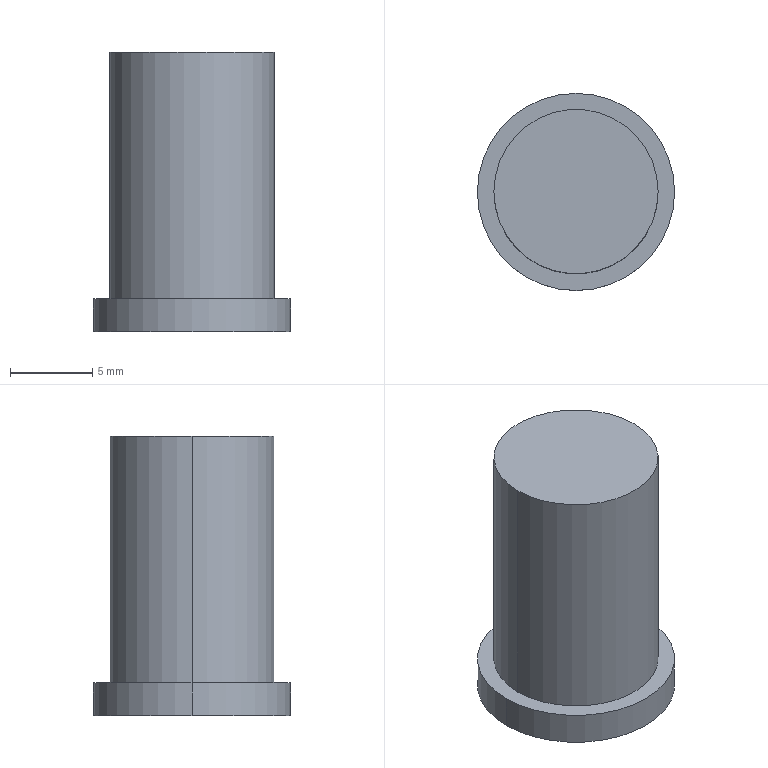Part | SolidWorks | features Extrusion 1, ICE 1 | 1 solid | 7 faces | box 12 x 12 x 17 mm | volume 1404 mm3 | cylinder 4 | plane 3 | commonest cylinder face diameters 10 x2 12 x2
STEP:
#1=CARTESIAN_POINT('',(5.,0.,17.));
#2=VERTEX_POINT('',#1);
#3=CARTESIAN_POINT('',(-5.,0.,17.));
#4=VERTEX_POINT('',#3);
#5=CARTESIAN_POINT('',(0.,0.,17.));
#6=DIRECTION('',(0.,0.,1.));
#7=DIRECTION('',(1.,0.,0.));
#8=AXIS2_PLACEMENT_3D('',#5,#6,#7);
#9=CIRCLE('',#8,5.);
#10=EDGE_CURVE('',#2,#4,#9,.T.);
#11=ORIENTED_EDGE('',*,*,#10,.F.);
#12=CARTESIAN_POINT('',(5.,0.,2.));
#13=VERTEX_POINT('',#12);
#14=CARTESIAN_POINT('',(5.,0.,17.));
#15=DIRECTION('',(0.,0.,-1.));
#16=VECTOR('',#15,1000.);
#17=LINE('',#14,#16);
#18=EDGE_CURVE('',#2,#13,#17,.T.);
#19=ORIENTED_EDGE('',*,*,#18,.T.);
#20=CARTESIAN_POINT('',(-5.,0.,2.));
#21=VERTEX_POINT('',#20);
#22=CARTESIAN_POINT('',(0.,0.,2.));
#23=DIRECTION('',(0.,0.,1.));
#24=DIRECTION('',(1.,0.,0.));
#25=AXIS2_PLACEMENT_3D('',#22,#23,#24);
#26=CIRCLE('',#25,5.);
#27=EDGE_CURVE('',#13,#21,#26,.T.);
#28=ORIENTED_EDGE('',*,*,#27,.T.);
#29=CARTESIAN_POINT('',(-5.,0.,17.));
#30=DIRECTION('',(0.,0.,-1.));
#31=VECTOR('',#30,1000.);
#32=LINE('',#29,#31);
#33=EDGE_CURVE('',#4,#21,#32,.T.);
#34=ORIENTED_EDGE('',*,*,#33,.F.);
#35=EDGE_LOOP('',(#11,#19,#28,#34));
#36=FACE_OUTER_BOUND('',#35,.T.);
#37=CARTESIAN_POINT('',(0.,0.,17.));
#38=DIRECTION('',(0.,0.,-1.));
#39=DIRECTION('',(-1.,0.,0.));
#40=AXIS2_PLACEMENT_3D('',#37,#38,#39);
#41=CYLINDRICAL_SURFACE('',#40,5.);
#42=ADVANCED_FACE('',(#36),#41,.T.);
#43=CARTESIAN_POINT('',(6.,0.,2.));
#44=VERTEX_POINT('',#43);
#45=CARTESIAN_POINT('',(-6.,0.,2.));
#46=VERTEX_POINT('',#45);
#47=CARTESIAN_POINT('',(0.,0.,2.));
#48=DIRECTION('',(0.,0.,1.));
#49=DIRECTION('',(1.,0.,0.));
#50=AXIS2_PLACEMENT_3D('',#47,#48,#49);
#51=CIRCLE('',#50,6.);
#52=EDGE_CURVE('',#44,#46,#51,.T.);
#53=ORIENTED_EDGE('',*,*,#52,.F.);
#54=CARTESIAN_POINT('',(6.,0.,0.));
#55=VERTEX_POINT('',#54);
#56=CARTESIAN_POINT('',(6.,0.,2.));
#57=DIRECTION('',(0.,0.,-1.));
#58=VECTOR('',#57,1000.);
#59=LINE('',#56,#58);
#60=EDGE_CURVE('',#44,#55,#59,.T.);
#61=ORIENTED_EDGE('',*,*,#60,.T.);
#62=CARTESIAN_POINT('',(-6.,0.,0.));
#63=VERTEX_POINT('',#62);
#64=CARTESIAN_POINT('',(0.,0.,0.));
#65=DIRECTION('',(0.,0.,1.));
#66=DIRECTION('',(1.,0.,0.));
#67=AXIS2_PLACEMENT_3D('',#64,#65,#66);
#68=CIRCLE('',#67,6.);
#69=EDGE_CURVE('',#55,#63,#68,.T.);
#70=ORIENTED_EDGE('',*,*,#69,.T.);
#71=CARTESIAN_POINT('',(-6.,0.,2.));
#72=DIRECTION('',(0.,0.,-1.));
#73=VECTOR('',#72,1000.);
#74=LINE('',#71,#73);
#75=EDGE_CURVE('',#46,#63,#74,.T.);
#76=ORIENTED_EDGE('',*,*,#75,.F.);
#77=EDGE_LOOP('',(#53,#61,#70,#76));
#78=FACE_OUTER_BOUND('',#77,.T.);
#79=CARTESIAN_POINT('',(0.,0.,2.));
#80=DIRECTION('',(0.,0.,-1.));
#81=DIRECTION('',(-1.,0.,0.));
#82=AXIS2_PLACEMENT_3D('',#79,#80,#81);
#83=CYLINDRICAL_SURFACE('',#82,6.);
#84=ADVANCED_FACE('',(#78),#83,.T.);
#85=ORIENTED_EDGE('',*,*,#60,.F.);
#86=CARTESIAN_POINT('',(0.,0.,2.));
#87=DIRECTION('',(0.,0.,1.));
#88=DIRECTION('',(1.,0.,0.));
#89=AXIS2_PLACEMENT_3D('',#86,#87,#88);
#90=CIRCLE('',#89,6.);
#91=EDGE_CURVE('',#46,#44,#90,.T.);
#92=ORIENTED_EDGE('',*,*,#91,.F.);
#93=ORIENTED_EDGE('',*,*,#75,.T.);
#94=CARTESIAN_POINT('',(0.,0.,0.));
#95=DIRECTION('',(0.,0.,1.));
#96=DIRECTION('',(1.,0.,0.));
#97=AXIS2_PLACEMENT_3D('',#94,#95,#96);
#98=CIRCLE('',#97,6.);
#99=EDGE_CURVE('',#63,#55,#98,.T.);
#100=ORIENTED_EDGE('',*,*,#99,.T.);
#101=EDGE_LOOP('',(#85,#92,#93,#100));
#102=FACE_OUTER_BOUND('',#101,.T.);
#103=CARTESIAN_POINT('',(0.,0.,2.));
#104=DIRECTION('',(0.,0.,-1.));
#105=DIRECTION('',(-1.,0.,0.));
#106=AXIS2_PLACEMENT_3D('',#103,#104,#105);
#107=CYLINDRICAL_SURFACE('',#106,6.);
#108=ADVANCED_FACE('',(#102),#107,.T.);
#109=CARTESIAN_POINT('',(0.,0.,2.));
#110=DIRECTION('',(0.,0.,1.));
#111=DIRECTION('',(1.,0.,0.));
#112=AXIS2_PLACEMENT_3D('',#109,#110,#111);
#113=CIRCLE('',#112,5.);
#114=EDGE_CURVE('',#21,#13,#113,.T.);
#115=ORIENTED_EDGE('',*,*,#114,.F.);
#116=ORIENTED_EDGE('',*,*,#27,.F.);
#117=EDGE_LOOP('',(#115,#116));
#118=FACE_BOUND('',#117,.T.);
#119=ORIENTED_EDGE('',*,*,#91,.T.);
#120=ORIENTED_EDGE('',*,*,#52,.T.);
#121=EDGE_LOOP('',(#119,#120));
#122=FACE_OUTER_BOUND('',#121,.T.);
#123=CARTESIAN_POINT('',(0.,0.,2.));
#124=DIRECTION('',(0.,0.,1.));
#125=DIRECTION('',(1.,0.,0.));
#126=AXIS2_PLACEMENT_3D('',#123,#124,#125);
#127=PLANE('',#126);
#128=ADVANCED_FACE('',(#118,#122),#127,.T.);
#129=ORIENTED_EDGE('',*,*,#99,.F.);
#130=ORIENTED_EDGE('',*,*,#69,.F.);
#131=EDGE_LOOP('',(#129,#130));
#132=FACE_OUTER_BOUND('',#131,.T.);
#133=CARTESIAN_POINT('',(0.,0.,0.));
#134=DIRECTION('',(0.,0.,1.));
#135=DIRECTION('',(1.,0.,0.));
#136=AXIS2_PLACEMENT_3D('',#133,#134,#135);
#137=PLANE('',#136);
#138=ADVANCED_FACE('',(#132),#137,.F.);
#139=ORIENTED_EDGE('',*,*,#18,.F.);
#140=CARTESIAN_POINT('',(0.,0.,17.));
#141=DIRECTION('',(0.,0.,1.));
#142=DIRECTION('',(1.,0.,0.));
#143=AXIS2_PLACEMENT_3D('',#140,#141,#142);
#144=CIRCLE('',#143,5.);
#145=EDGE_CURVE('',#4,#2,#144,.T.);
#146=ORIENTED_EDGE('',*,*,#145,.F.);
#147=ORIENTED_EDGE('',*,*,#33,.T.);
#148=ORIENTED_EDGE('',*,*,#114,.T.);
#149=EDGE_LOOP('',(#139,#146,#147,#148));
#150=FACE_OUTER_BOUND('',#149,.T.);
#151=CARTESIAN_POINT('',(0.,0.,17.));
#152=DIRECTION('',(0.,0.,-1.));
#153=DIRECTION('',(-1.,0.,0.));
#154=AXIS2_PLACEMENT_3D('',#151,#152,#153);
#155=CYLINDRICAL_SURFACE('',#154,5.);
#156=ADVANCED_FACE('',(#150),#155,.T.);
#157=ORIENTED_EDGE('',*,*,#145,.T.);
#158=ORIENTED_EDGE('',*,*,#10,.T.);
#159=EDGE_LOOP('',(#157,#158));
#160=FACE_OUTER_BOUND('',#159,.T.);
#161=CARTESIAN_POINT('',(0.,0.,17.));
#162=DIRECTION('',(0.,0.,1.));
#163=DIRECTION('',(1.,0.,0.));
#164=AXIS2_PLACEMENT_3D('',#161,#162,#163);
#165=PLANE('',#164);
#166=ADVANCED_FACE('',(#160),#165,.T.);
#167=CLOSED_SHELL('',(#42,#84,#108,#128,#138,#156,#166));
#168=MANIFOLD_SOLID_BREP('',#167);
#169=CARTESIAN_POINT('',(0.,0.,0.));
#170=DIRECTION('',(0.,0.,1.));
#171=DIRECTION('',(1.,0.,0.));
#172=AXIS2_PLACEMENT_3D('',#169,#170,#171);
#173=(LENGTH_UNIT()NAMED_UNIT(*)SI_UNIT(.MILLI.,.METRE.));
#174=UNCERTAINTY_MEASURE_WITH_UNIT(LENGTH_MEASURE(0.00001),#173,'','');
#175=(NAMED_UNIT(*)PLANE_ANGLE_UNIT()SI_UNIT($,.RADIAN.));
#176=(NAMED_UNIT(*)SI_UNIT($,.STERADIAN.)SOLID_ANGLE_UNIT());
#177=(GEOMETRIC_REPRESENTATION_CONTEXT(3)GLOBAL_UNCERTAINTY_ASSIGNED_CONTEXT((#174))GLOBAL_UNIT_ASSIGNED_CONTEXT((#173,#175,#176))REPRESENTATION_CONTEXT('',''));
#178=ADVANCED_BREP_SHAPE_REPRESENTATION('',(#168,#172),#177);